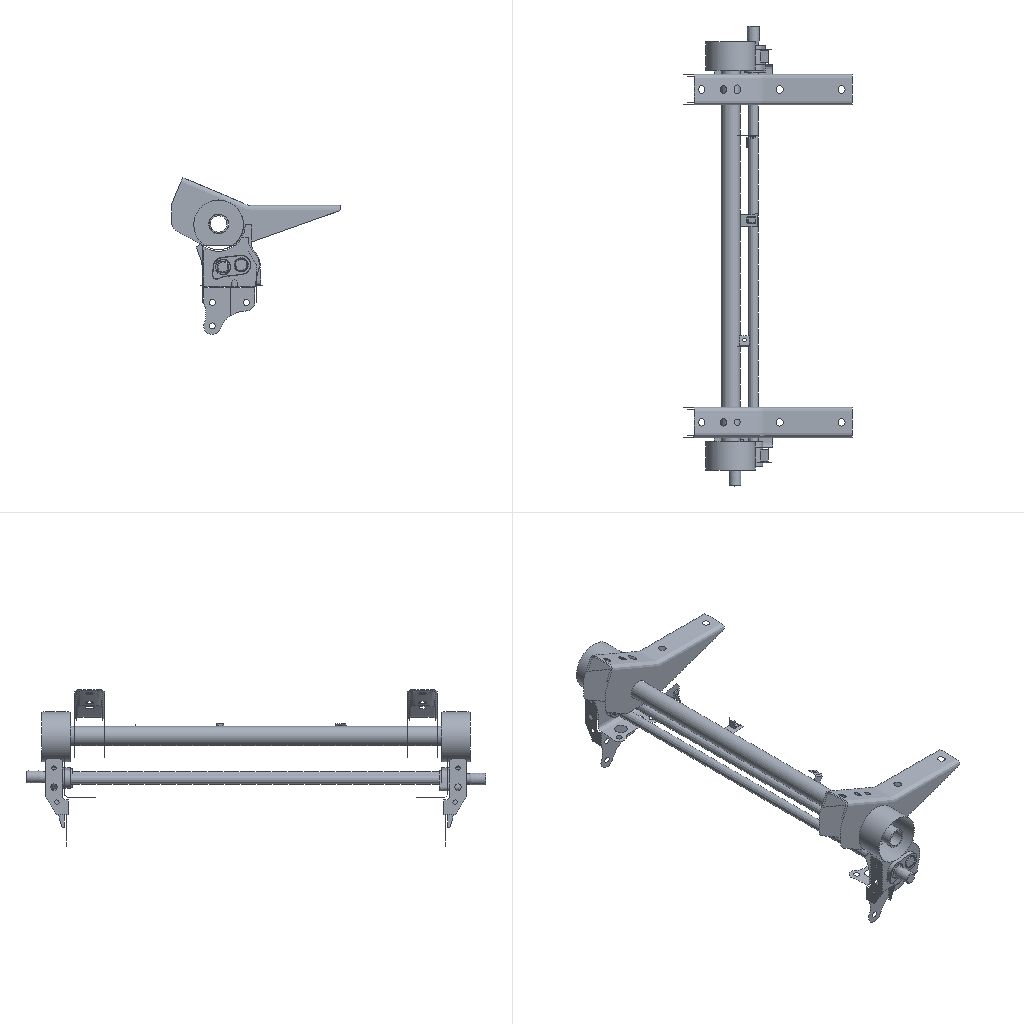Simulation study | nastran
Set-up summary:
category,name,step,type,value,unit,region
solver,nx_nastran
units,not stated in the deck,,not stated
analysis,deck,,static,static
analysis,solution,,SOL,101
load_step,SUBCASE 2,2,SUBCASE,SPC=1 LOAD=3
load_step,SUBCASE 3,3,SUBCASE,SPC=1 LOAD=4
load_step,SUBCASE 4,4,SUBCASE,SPC=1 LOAD=5
load_step,requested,,,3
mesh,nodes,,,50435
mesh,elements,,,150385
element_type,CQUAD4,,shell,13466
element_type,CTETRA,,solid,136311
element_type,CTRIA3,,shell,608
load,load commands in deck,,count,3
bc,support commands in deck,,count,10
check,setup vs results,,match,"every grid point's frame and coordinates and every element id; grid points of CQUAD4, CTETRA, CTRIA3 elements"
Nastran input file, long lists of numbers shortened:
$$------------------------------------------------------------------------------$
$$                                                                              $
$$ NASTRAN Input Deck Generated by HyperMesh Version  : 9.0b121                 $
$$ Generated using HyperMesh-Nastran Template Version : 9.0b121
$$                                                                              $
$$   Template:  general                                                         $
$$                                                                              $
$$------------------------------------------------------------------------------$
$$------------------------------------------------------------------------------$
$$                      Executive Control Cards                                 $
$$------------------------------------------------------------------------------$
SOL 101
CEND
$$------------------------------------------------------------------------------$
$$                      Case Control Cards                                      $
$$------------------------------------------------------------------------------$
  DISPLACEMENT = ALL
$
$HMNAME LOADSTEP               2"LOADX"
SUBCASE       2
  LABEL= LOADX
  SPC =        1
  LOAD =        3
$
$HMNAME LOADSTEP               3"LOADY"
SUBCASE       3
  LABEL= LOADY
  SPC =        1
  LOAD =        4
$
$HMNAME LOADSTEP               4"LOADZ"
SUBCASE       4
  LABEL= LOADZ
  SPC =        1
  LOAD =        5
$$------------------------------------------------------------------------------$
$$                      Bulk Data Cards                                         $
$$------------------------------------------------------------------------------$
BEGIN BULK
PARAM,POST,-1
$$
$$  GRID Data
$$
GRID        1878        -1076.71-453.0  -46.8081
GRID        1879        -1075.89-453.0  -44.0031
$ (50433 more lines like these left out)
$$
$$  SPOINT Data
$$
$$
$$------------------------------------------------------------------------------$
$$             Group Definitions                                                $
$$------------------------------------------------------------------------------$
$
$ RBE2 Elements - Single dependent node
$
RBE2      319319   31735  123456   33228
RBE2      319320   31734  123456   33241
$ (427 more lines like these left out)
$
$HMMOVE       17
$         319319THRU      319321  319323THRU      319326  319328THRU      319354
$         319373THRU      319377  319379THRU      319380  319383THRU      319386
$ (27 more lines like these left out)
RBE2      319322   33239  123456   31731   31732
RBE2      319355   31878  123456   33636   33637
$ (1231 more lines like these left out)
$
$HMMOVE       17
$         319322  319355THRU      319372  319378  319381THRU      319382  319387
$         319400THRU      319401  319405  319407THRU      319410  319412  319414
$ (28 more lines like these left out)
CTRIA3     78851       2   20757   20758   20756
CTRIA3     78880       2   20783   20784   20811
$ (606 more lines like these left out)
$
$HMMOVE        2
$          78851   78880   78885   78888   78898   78914   78927   78932   78948
$          78953   78958   78975   79006   79278   79303   79305THRU       79306
$ (100 more lines like these left out)
CQUAD4     78172       2   19798   19799   19772   19773
CQUAD4     78173       2   19799   19800   19771   19772
$ (13464 more lines like these left out)
$
$HMMOVE        2
$          78172THRU       78850   78852THRU       78879   78881THRU       78884
$          78886THRU       78887   78889THRU       78897   78899THRU       78913
$ (210 more lines like these left out)
CTETRA     33446      10   12354   10779   10738   10739
CTETRA     33447      10   11713   10206   10272   10268
$ (136309 more lines like these left out)
$
$HMMOVE        6
$          33446THRU       34445   32446THRU       33445   31446THRU       32445
$          25804THRU       25880   30523THRU       31445   29523THRU       30522
$ (77 more lines like these left out)
PSHELL         2       14.5            1               1
$
$HMNAME PROP                   3"100" 4
$HWCOLOR PROP                  3       5
PSHELL         3       110.0           1               1
$
$HMNAME PROP                   4"60" 4
$HWCOLOR PROP                  4       6
PSHELL         4       16.0            1               1
$
$HMNAME PROP                   5"20" 4
$HWCOLOR PROP                  5       7
PSHELL         5       12.0            1               1
$
$HMNAME PROP                   6"12" 4
$HWCOLOR PROP                  6       8
PSHELL         6       11.2            1               1
$
$HMNAME PROP                   7"15" 4
$HWCOLOR PROP                  7       9
PSHELL         7       11.5            1               1
$
$HMNAME PROP                   8"2.2" 4
$HWCOLOR PROP                  8      13
PSHELL         8       12.2            1               1
$
$HMNAME PROP                   9"55" 4
$HWCOLOR PROP                  9      17
PSHELL         9       15.5            1               1
$$
$$  PSOLID Data
$
$HMNAME PROP                  10"solid" 5
$HWCOLOR PROP                 10      20
PSOLID        10       1
$$
$$  PBUSH Data
$
$HMNAME PROP                   1"bush"
$HWCOLOR PROP                  1       3
PBUSH          1       K10000.0 10000.0 10000.0 10000.0 1.0     10000.0
$$
$$------------------------------------------------------------------------------$
$$                      Material Definition Cards                               $
$$------------------------------------------------------------------------------$
$$--------------------------------------------------------------
$$ HYPERMESH TAGS
$$--------------------------------------------------------------
$$BEGIN TAGS
$$END TAGS
$$
$$  MAT1 Data
$
$HMNAME MAT                    1"steel" "MAT1"
$HWCOLOR MAT                   1       3
MAT1           1210000.0        0.3     7.85E-09
$$
$$
$$
$$------------------------------------------------------------------------------$
$ (43 more lines like these left out)
SPC            1   63138  1234560.0
SPC            1   63139  1234560.0
SPC            1   63140  1234560.0
SPC            1   63141  1234560.0
SPC            1   63142  1234560.0
SPC            1   63143  1234560.0
SPC            1   63144  1234560.0
SPC            1   63145  1234560.0
SPC            1   63146  1234560.0
SPC            1   63147  1234560.0
$$
$$  FORCE Data
$$
FORCE          3   63148       01.0     1000.0  0.0     0.0
FORCE          4   63148       01.0     0.0     1000.0  0.0
FORCE          5   63148       01.0     0.0     0.0     1000.0
$HMASSEM       1       3 5002500LG010
$HMASSEM_ASSEM_ID              2
$HMASSEM       2       4 5002500LG010.1
$
ENDDATA
Results summary:
result,analysis,,,static
result,last_loadstep,,,3
result,primary field,,,displacements
result,max displacement,,,0.04396,model units